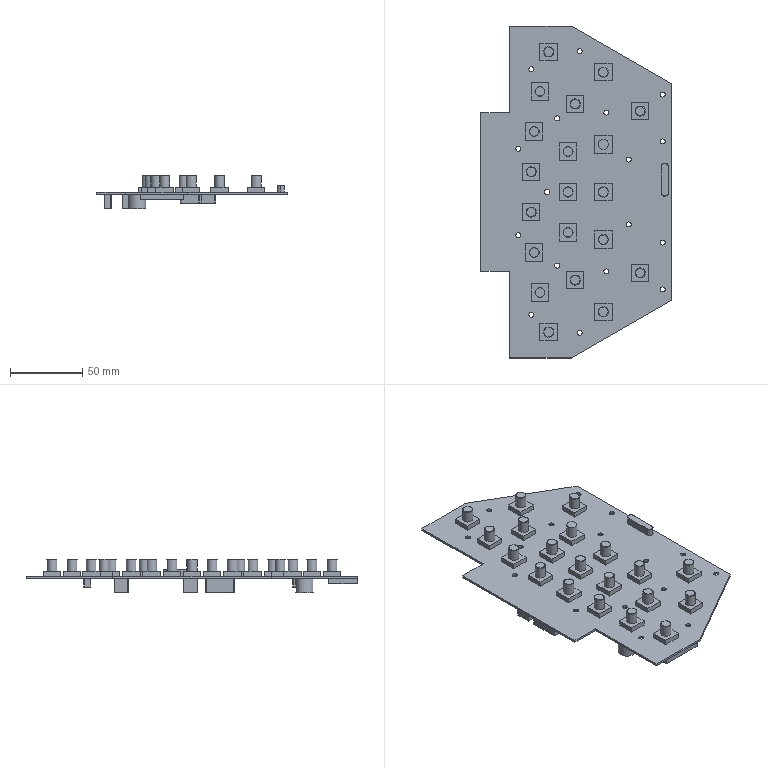Part | STEP file | PCB Plate-618 | 1 solid | 268 faces | box 132 x 230 x 23.4 mm | volume 58668 mm3 | plane 201 | cylinder 44 | torus 23 | commonest cylinder face diameters 7 x20 3.5 x17 5 x4 0.4 x2 12.12 x1